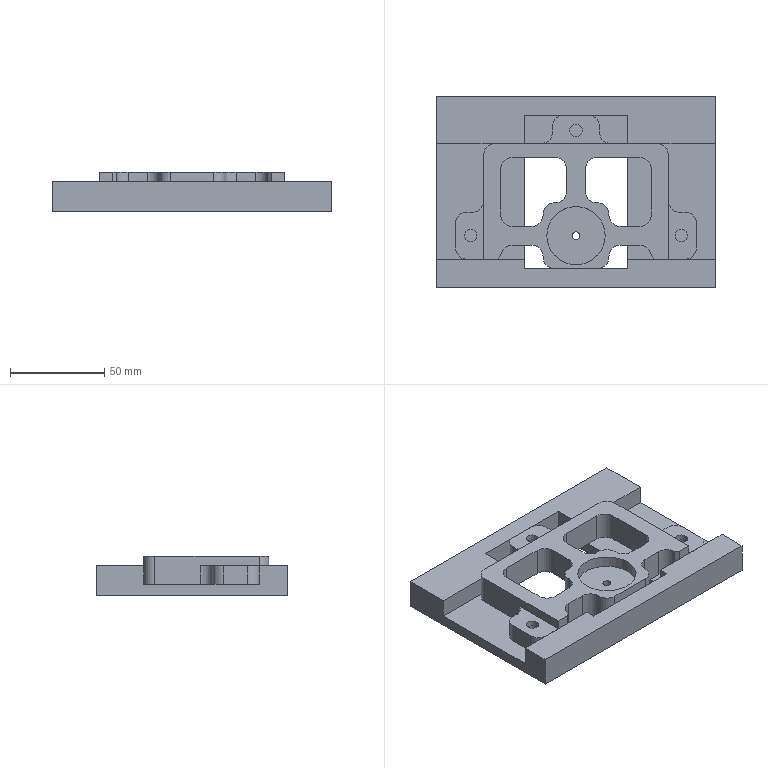NC program | NX | posted with a generic post | part box 148 x 101.5 x 21 mm
Lines 5225 to 5700 of 5700:
(ZLEVEL_PROFILE_COPY , TOOL : D10JING)
N10406 T14 M6
N10408 G54
N10410 G17 G0 G90 X34. Y-12.25 S9500 M3
N10412 G43 Z30. H14
N10414 Z-21.
N10416 G94 G1 X34.5 Y-13.116 F1000.
N10418 G3 X35. Y-12.25 R1.
N10420 G1 Y12.25 F1200.
N10422 G3 X34. Y13.25 R1.
N10424 G1 X23.5
N10426 G3 X22.5 Y12.25 R1.
N10428 G1 Y11.75
N10430 G2 X11.5 Y0.75 R11.
N10432 G1 X11.
N10434 G3 X10. Y-0.25 R1.
N10436 G1 Y-12.25
N10438 G3 X11. Y-13.25 R1.
N10440 G1 X34.
N10442 G3 X35. Y-12.25 R1.
N10444 X34.5 Y-11.384 R1.
N10446 G1 X34. Y-11.095
N10448 G0 Z30.
N10450 X-34. Y-12.25
N10452 Z-21.
N10454 G1 X-34.866 Y-12.75 F1000.
N10456 G3 X-34. Y-13.25 R1.
N10458 G1 X-11. F1200.
N10460 G3 X-10. Y-12.25 R1.
N10462 G1 Y-0.25
N10464 G3 X-11. Y0.75 R1.
N10466 G1 X-11.5
N10468 G2 X-22.5 Y11.75 R11.
N10470 G1 Y12.25
N10472 G3 X-23.5 Y13.25 R1.
N10474 G1 X-34.
N10476 G3 X-35. Y12.25 R1.
N10478 G1 Y-12.25
N10480 G3 X-34. Y-13.25 R1.
N10482 X-33.134 Y-12.75 R1.
N10484 G1 X-32.845 Y-12.25
N10486 G0 Z30.
(FLOOR_WALL_COPY_COPY , TOOL : D10JING)
N10488 X-71.823 Y14.534
N10490 Z-2.
N10492 G1 Z-5. F1000.
N10494 X-69.5 Y15.875
N10496 G3 X-69. Y16.741 R1.
N10498 G1 Y29.759
N10500 G2 X-64.167 Y38.859 R11.
N10502 G1 Y7.641
N10504 G3 X-59.333 Y5.831 R11.
N10506 G1 Y40.669
N10508 G2 X-58. Y40.75 R11.
N10510 G1 X-54.5
N10512 Y5.616
N10514 G2 X-55. Y4.75 R1.
N10516 G1 X-58.451 Y2.757
N10518 Z-2.
N10520 X-57. Y2.687 F8000.
N10522 Z-5. F1000.
N10524 X-54.5 Y4.131
N10526 G3 X-54. Y4.997 R1.
N10528 G1 Y40.75
N10530 G3 X-54.5 Y41.616 R1.
N10532 G1 X-58.194 Y43.749
N10534 Z-2.
N10536 G0 Z30.
N10538 X8.72 Y-48.573
N10540 Z-2.
N10542 G1 Z-5.
N10544 X7.379 Y-46.25
N10546 G3 X6.513 Y-45.75 R1.
N10548 G1 X-6.513
N10550 G2 X-15.609 Y-40.917 R11.
N10552 G1 X15.609
N10554 G3 X17.419 Y-36.083 R11.
N10556 G1 X-17.419
N10558 X-17.48 Y-35.418
N10560 X-17.634 Y-31.25
N10562 X17.634
N10564 G2 X18.5 Y-31.75 R1.
N10566 G1 X20.493 Y-35.202
N10568 Z-2.
N10570 X20.563 Y-33.75 F8000.
N10572 Z-5. F1000.
N10574 X19.119 Y-31.25
N10576 G3 X18.253 Y-30.75 R1.
N10578 G1 X-18.253
N10580 G3 X-19.119 Y-31.25 R1.
N10582 G1 X-20.563 Y-33.75
N10584 Z-2.
N10586 G0 Z30.
N10588 X45.284 Y-33.562
N10590 Z3.
N10592 G1 Z0.
N10594 X43.948 Y-31.25
N10596 G3 X43.082 Y-30.75 R1.
N10598 G1 X35.862
N10600 X-43.
N10602 G2 X-52.098 Y-25.932 R11.
N10604 G1 X52.101 Y-25.928
N10606 G3 X53.916 Y-21.106 R11.
N10608 G1 X-53.916 Y-21.111
N10610 G2 X-54. Y-19.75 R11.
N10612 G1 Y-16.289
N10614 X54. Y-16.285
N10616 Y-11.463
N10618 X35. Y-11.464
N10620 Y-6.642
N10622 X54. Y-6.641
N10624 Y-1.82
N10626 X35. Y-1.821
N10628 Y3.001
N10630 X54. Y3.002
N10632 Y7.823
N10634 X35. Y7.822
N10636 X34.919 Y12.644
N10638 X54. Y12.645
N10640 G2 X54.866 Y12.145 R1.
N10642 G1 X57. Y8.449
N10644 Z3.
N10646 X13. Y-10.25 F8000.
N10648 Z0. F1000.
N10650 X10.866 Y-11.965
N10652 G3 X10. Y-11.465 R1.
N10654 G1 X-10. Y-11.466
N10656 Y-6.644
N10658 X10. Y-6.643
N10660 Y-1.822
N10662 X-10. Y-1.823
N10664 X-16.972 Y2.208
N10666 X-18.164 Y2.999
N10668 X18.166 Y3.
N10670 G3 X21.775 Y7.822 R11.
N10672 G1 X-21.774 Y7.82
N10674 X-22.175 Y9.097
N10676 X-22.419 Y10.414
N10678 X-22.58 Y12.641
N10680 X22.581 Y12.643
N10682 G2 X23.447 Y12.143 R1.
N10684 G1 X25.236 Y9.044
N10686 Z3.
N10688 X-32. Y-10.25 F8000.
N10690 Z0. F1000.
N10692 X-34.134 Y-11.967
N10694 G3 X-35. Y-11.467 R1.
N10696 G1 X-54. Y-11.468
N10698 Y-6.646
N10700 X-35. Y-6.645
N10702 Y-1.824
N10704 X-54. Y-1.825
N10706 Y2.997
N10708 X-35. Y2.998
N10710 Y7.819
N10712 X-54.
N10714 Y12.64
N10716 X-34.92 Y12.641
N10718 X54. Y17.466
N10720 X8.762 Y17.464
N10722 X10.456 Y22.286
N10724 X54. Y22.288
N10726 Y27.109
N10728 X9.766 Y27.108
N10730 X5.91 Y31.929
N10732 X54. Y31.931
N10734 G2 X54.866 Y31.431 R1.
N10736 G1 X57. Y27.735
N10738 Z3.
N10740 X-5.867 Y18.578 F8000.
N10742 Z0. F1000.
N10744 X-7.896 Y16.964
N10746 G3 X-8.762 Y17.464 R1.
N10748 G1 X-54. Y17.462
N10750 Y22.283
N10752 X-10.456 Y22.285
N10754 X-9.766 Y27.107
N10756 X-54. Y27.105
N10758 Y31.926
N10760 X-5.911 Y31.928
N10762 X22.316 Y36.751
N10764 X-22.317 Y36.749
N10766 G3 X-23.183 Y36.249 R1.
N10768 G1 X-25.386 Y36.532
N10770 Z3.
N10772 G0 Z30.
N10774 X-0.859 Y13.749
N10776 Z-3.
N10778 G1 Z-6.
N10780 G3 X0.008 Y13.25 R1.
N10782 G1 X-0.007
N10784 G2 X-8.66 Y18.25 R10.
N10786 G1 X8.66
N10788 G3 X10. Y23.25 R10.
N10790 G1 X-10.
N10792 G2 X-8.66 Y28.25 R10.
N10794 G1 X8.66
N10796 G3 X0.007 Y33.25 R10.
N10798 G1 X-0.008
N10800 G3 X-0.874 Y32.75 R1.
N10802 G1 X0.858 Y33.251
N10804 G3 X-0.008 Y33.75 R1.
N10806 X-10.5 Y23.242 R10.5
N10808 X-0.008 Y33.75 R-10.5
N10810 X-0.874 Y33.249 R1.
N10812 G1 X-2.577 Y30.293
N10814 Z-3.
N10816 G0 Z30.
N10818 X71.823 Y31.969
N10820 Z-2.
N10822 G1 Z-5.
N10824 X69.5 Y30.628
N10826 G3 X69. Y29.762 R1.
N10828 G1 Y16.738
N10830 G2 X64.167 Y7.641 R11.
N10832 G1 Y38.859
N10834 G3 X59.333 Y40.669 R11.
N10836 G1 Y5.831
N10838 X58.668 Y5.77
N10840 X54.5 Y5.616
N10842 Y40.75
N10844 G2 X55. Y41.616 R1.
N10846 G1 X58.668 Y43.734
N10848 Z-2.
N10850 X58.194 Y43.749 F8000.
N10852 Z-5. F1000.
N10854 X54.5 Y41.616
N10856 G3 X54. Y40.75 R1.
N10858 G1 Y4.997
N10860 G3 X54.5 Y4.131 R1.
N10862 G1 X57. Y2.687
N10864 Z-2.
N10866 G0 Z30.
(ZLEVEL_PROFILE_COPY_COPY , TOOL : D10JING)
N10868 X55. Y4.75
N10870 Z-21.
N10872 G1 X54.5 Y5.616
N10874 G3 X54. Y4.75 R1.
N10876 G1 Y-19.75 F1200.
N10878 G2 X43. Y-30.75 R11.
N10880 G1 X18.5
N10882 G3 X17.5 Y-31.75 R1.
N10884 G1 Y-34.75
N10886 G2 X6.5 Y-45.75 R11.
N10888 G1 X-6.5
N10890 G2 X-17.5 Y-34.75 R11.
N10892 G1 Y-31.75
N10894 G3 X-18.5 Y-30.75 R1.
N10896 G1 X-43.
N10898 G2 X-54. Y-19.75 R11.
N10900 G1 Y4.75
N10902 G3 X-55. Y5.75 R1.
N10904 G1 X-58.
N10906 G2 X-69. Y16.75 R11.
N10908 G1 Y29.75
N10910 G2 X-58. Y40.75 R11.
N10912 G1 X-41.984
N10914 G2 X-38.561 Y39.394 R5.
N10916 G1 X-36.565 Y37.519
N10918 G2 X-34.998 Y34.188 R5.
N10920 G3 X-34. Y33.25 R1.
N10922 G1 X-23.5
N10924 G3 X-22.5 Y34.25 R1.
N10926 G1 Y34.75
N10928 G2 X-11.5 Y45.75 R11.
N10930 G1 X11.5
N10932 G2 X22.5 Y34.75 R11.
N10934 G1 Y34.25
N10936 G3 X23.5 Y33.25 R1.
N10938 G1 X34.
N10940 G3 X34.998 Y34.188 R1.
N10942 G2 X36.565 Y37.519 R5.
N10944 G1 X38.561 Y39.394
N10946 G2 X41.984 Y40.75 R5.
N10948 G1 X58.
N10950 G2 X69. Y29.75 R11.
N10952 G1 Y16.75
N10954 G2 X58. Y5.75 R11.
N10956 G1 X55.
N10958 G3 X54. Y4.75 R1.
N10960 X54.5 Y3.884 R1.
N10962 G1 X55. Y3.595
N10964 G0 Z30.
N10966 M5
(ZLEVEL_PROFILE_1 , TOOL : D6A45)
N10968 T01 M6
N10970 G54
N10972 G17 G0 G90 X-23.539 Y-15.841 S9500 M3
N10974 G43 Z30. H1
N10976 Z0.25
N10978 G94 G1 Z-1.25 F1250.
N10980 X-23.02 Y-16.741
N10982 G3 X-22.5 Y-17.041 R0.6
N10984 G1 X-11.
N10986 G3 X-6.209 Y-12.25 R4.791
N10988 G1 Y-0.25
N10990 G3 X-11. Y4.541 R4.791
N10992 G1 X-11.5
N10994 G2 X-18.709 Y11.75 R7.209
N10996 G1 Y12.25
N10998 G3 X-23.5 Y17.041 R4.791
N11000 G1 X-34.
N11002 G3 X-38.791 Y12.25 R4.791
N11004 G1 Y-12.25
N11006 G3 X-34. Y-17.041 R4.791
N11008 G1 X-22.5
N11010 G3 X-21.98 Y-16.741 R0.6
N11012 G1 X-21.461 Y-15.841
N11014 Z0.25
N11016 G0 Z30.
N11018 X21.461
N11020 Z0.25
N11022 G1 Z-1.25
N11024 X21.98 Y-16.741
N11026 G3 X22.5 Y-17.041 R0.6
N11028 G1 X34.
N11030 G3 X38.791 Y-12.25 R4.791
N11032 G1 Y12.25
N11034 G3 X34. Y17.041 R4.791
N11036 G1 X23.5
N11038 G3 X18.709 Y12.25 R4.791
N11040 G1 Y11.75
N11042 G2 X11.5 Y4.541 R7.209
N11044 G1 X11.
N11046 G3 X6.209 Y-0.25 R4.791
N11048 G1 Y-12.25
N11050 G3 X11. Y-17.041 R4.791
N11052 G1 X22.5
N11054 G3 X23.02 Y-16.741 R0.6
N11056 G1 X23.539 Y-15.841
N11058 Z0.25
N11060 G0 Z30.
N11062 X1.064 Y36.298
N11064 Z0.25
N11066 G1 Z-1.25
N11068 X0.52 Y37.241
N11070 G3 X0. Y37.541 R0.6
N11072 X-14.291 Y23.25 R14.291
N11074 X0. Y37.541 R-14.291
N11076 X-0.52 Y37.241 R0.6
N11078 G1 X-1.064 Y36.298
N11080 Z0.25
N11082 G0 Z30.
N11084 X1.039 Y-28.159
N11086 Z0.25
N11088 G1 Z-1.25
N11090 X0.52 Y-27.259
N11092 G3 X0. Y-26.959 R0.6
N11094 G1 X-43.
N11096 G2 X-50.209 Y-19.75 R7.209
N11098 G1 Y35.759
N11100 G2 X-49.003 Y36.959 R1.202
N11102 G1 X-41.983
N11104 G2 X-41.159 Y36.633 R1.203
N11106 G1 X-39.159 Y34.754
N11108 G2 X-38.782 Y33.953 R1.201
N11110 G3 X-34. Y29.459 R4.791
N11112 G1 X-23.5
N11114 G3 X-18.709 Y34.25 R4.791
N11116 G1 Y34.75
N11118 G2 X-11.5 Y41.959 R7.209
N11120 G1 X11.5
N11122 G2 X18.709 Y34.75 R7.209
N11124 G1 Y34.25
N11126 G3 X23.5 Y29.459 R4.791
N11128 G1 X34.
N11130 G3 X38.782 Y33.953 R4.791
N11132 G2 X39.159 Y34.754 R1.201
N11134 G1 X41.159 Y36.633
N11136 G2 X41.983 Y36.959 R1.203
N11138 G1 X49.003
N11140 G2 X50.209 Y35.759 R1.202
N11142 G1 Y-19.75
N11144 G2 X43. Y-26.959 R7.209
N11146 G1 X0.
N11148 G3 X-0.52 Y-27.259 R0.6
N11150 G1 X-1.039 Y-28.159
N11152 Z0.25
N11154 G0 Z30.
N11156 X15.153 Y-29.85
N11158 Z-4.5
N11160 G1 Z-6.
N11162 X14.372 Y-29.099
N11164 G3 X14.113 Y-29.25 R0.3
N11166 X13.451 Y-31.75 R5.049
N11168 G1 Y-34.75
N11170 G2 X6.5 Y-41.701 R6.951
N11172 G1 X-6.5
N11174 G2 X-13.451 Y-34.75 R6.951
N11176 G1 Y-31.75
N11178 G3 X-14.113 Y-29.25 R5.049
N11180 X-14.372 Y-29.099 R0.3
N11182 G1 X-15.153 Y-29.85
N11184 Z-4.5
N11186 G0 Z30.
N11188 X-53.1 Y8.097
N11190 Z-4.5
N11192 G1 Z-6.
N11194 X-52.364 Y8.887
N11196 G3 X-52.516 Y9.146 R0.3
N11198 X-55. Y9.799 R5.049
N11200 G1 X-58.
N11202 G2 X-64.951 Y16.75 R6.951
N11204 G1 Y29.75
N11206 G2 X-58. Y36.701 R6.951
N11208 G1 X-52.398
N11210 G3 X-52.139 Y36.851 R0.3
N11212 G1 X-52.49 Y37.901
N11214 Z-4.5
N11216 G0 Z30.
N11218 X52.49
N11220 Z-4.5
N11222 G1 Z-6.
N11224 X52.139 Y36.851
N11226 G3 X52.398 Y36.701 R0.3
N11228 G1 X58.
N11230 G2 X64.951 Y29.75 R6.951
N11232 G1 Y16.75
N11234 G2 X58. Y9.799 R6.951
N11236 G1 X55.
N11238 G3 X52.516 Y9.146 R5.049
N11240 X52.364 Y8.887 R0.3
N11242 G1 X53.1 Y8.097
N11244 Z-4.5
N11246 G0 Z30.
N11248 X-0.282 Y-33.864
N11250 Z-4.5
N11252 G1 Z-6.
N11254 X-0.52 Y-34.799
N11256 G3 X0. Y-35.099 R0.6
N11258 X2.349 Y-32.75 R2.349
N11260 X0. Y-35.099 R-2.349
N11262 X0.52 Y-34.799 R0.6
N11264 G1 X0.282 Y-33.864
N11266 Z-4.5
N11268 G0 Z30.
N11270 X-57.114 Y23.532
N11272 Z-4.5
N11274 G1 Z-6.
N11276 X-58.049 Y23.77
N11278 G3 X-58.349 Y23.25 R0.6
N11280 X-56. Y20.901 R2.349
N11282 X-58.349 Y23.25 R-2.349
N11284 X-58.049 Y22.73 R0.6
N11286 G1 X-57.114 Y22.968
N11288 Z-4.5
N11290 G0 Z30.
N11292 X57.114
N11294 Z-4.5
N11296 G1 Z-6.
N11298 X58.049 Y22.73
N11300 G3 X58.349 Y23.25 R0.6
N11302 X56. Y25.599 R2.349
N11304 X58.349 Y23.25 R-2.349
N11306 X58.049 Y23.77 R0.6
N11308 G1 X57.114 Y23.532
N11310 Z-4.5
N11312 G0 Z30.
N11314 X0. Y23.891
N11316 Z-4.5
N11318 G1 Z-7.5
N11320 G3 X-0.641 Y23.25 R0.641
N11322 X0. Y23.891 R-0.641
N11324 X-0.52 Y23.591 R0.6
N11326 G1 Z-6.
N11328 G0 Z30.
N11330 M5
N11332 M2